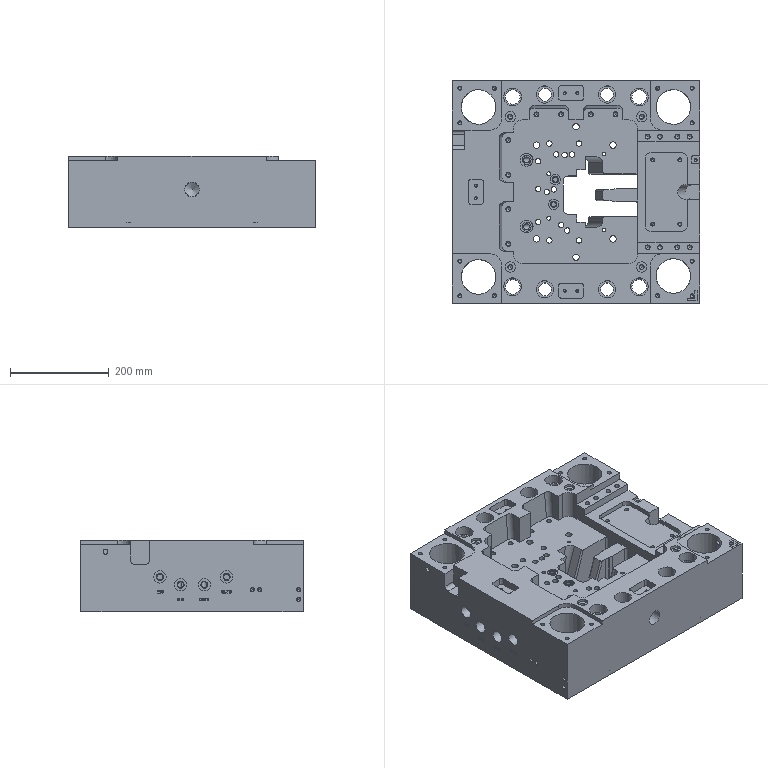Part | STEP file | BB | 1 solid | 632 faces | box 500 x 450 x 145 mm | volume 21236141 mm3 | plane 305 | cylinder 239 | cone 61 | other 27 | commonest cylinder face diameters 10 x41 8 x26 6.7 x24 8.5 x16 20 x16 11 x14